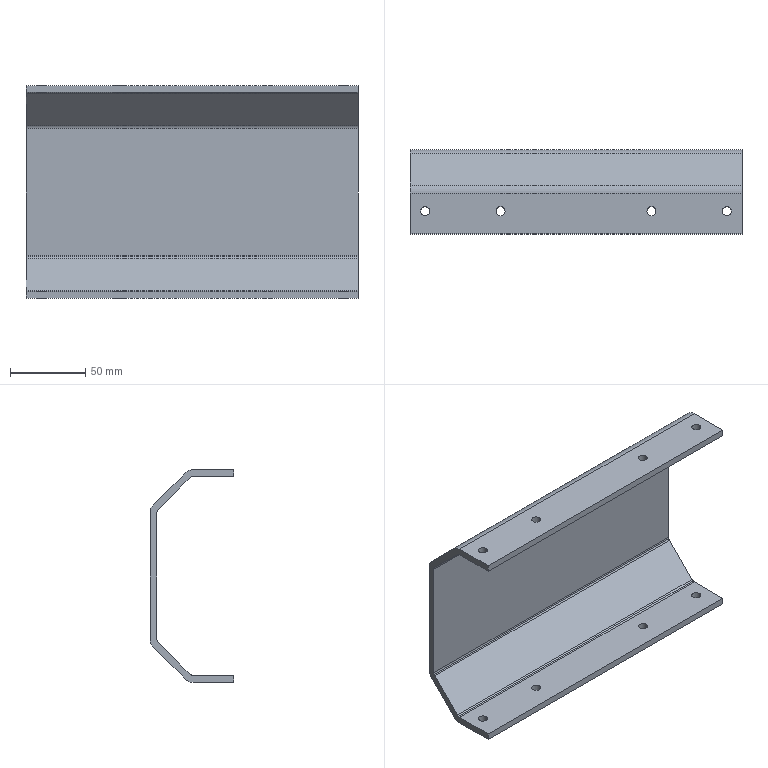Part | STEP file | JOINT.BRACKET.stp | 1 solid | 42 faces | box 220 x 55.5 x 141 mm | volume 210609 mm3 | spline 20 | cylinder 16 | plane 6 | commonest cylinder face diameters 6 x12 15 x4